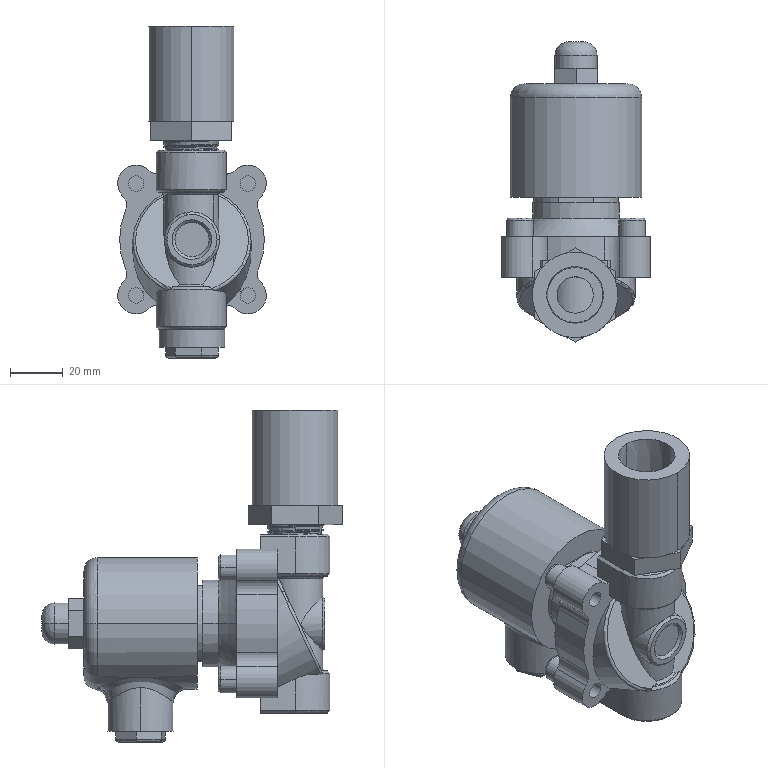Part | SolidWorks | 12 solids | 363 faces | box 56.5 x 114.123 x 126.119 mm | volume 204524 mm3 | cylinder 161 | plane 110 | spline 49 | cone 31 | torus 12 | commonest cylinder face diameters 19.583 x40 18.5 x37 45 x17 10 x16 6 x8 2 x6